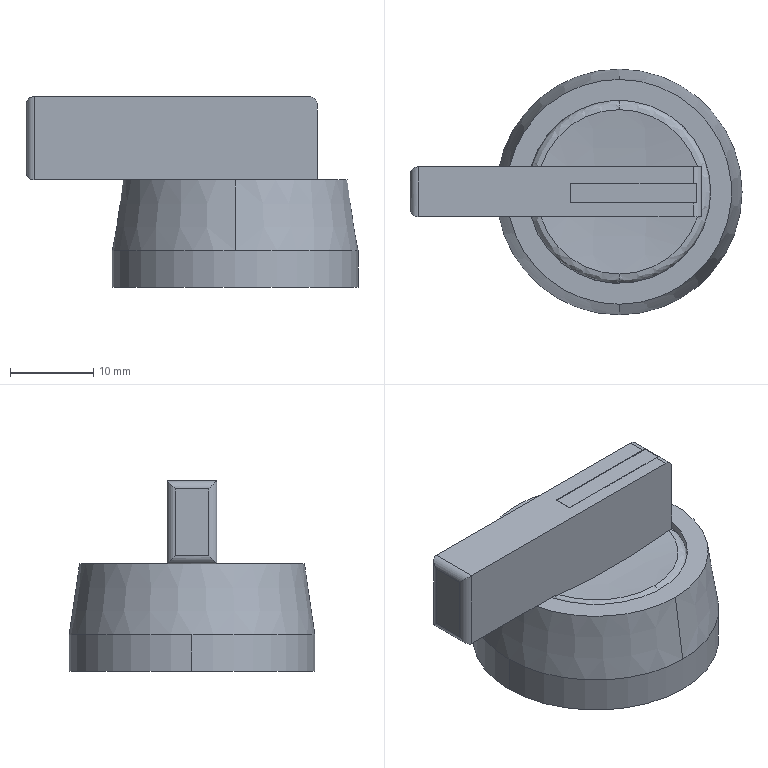Part | STEP file | LAY8_1-1_1 | 1 solid | 33 faces | box 39.873 x 29.5 x 22.9 mm | volume 10327 mm3 | plane 14 | cylinder 13 | spline 4 | cone 2 | commonest cylinder face diameters 2 x5 160 x4 22 x2 29.5 x2